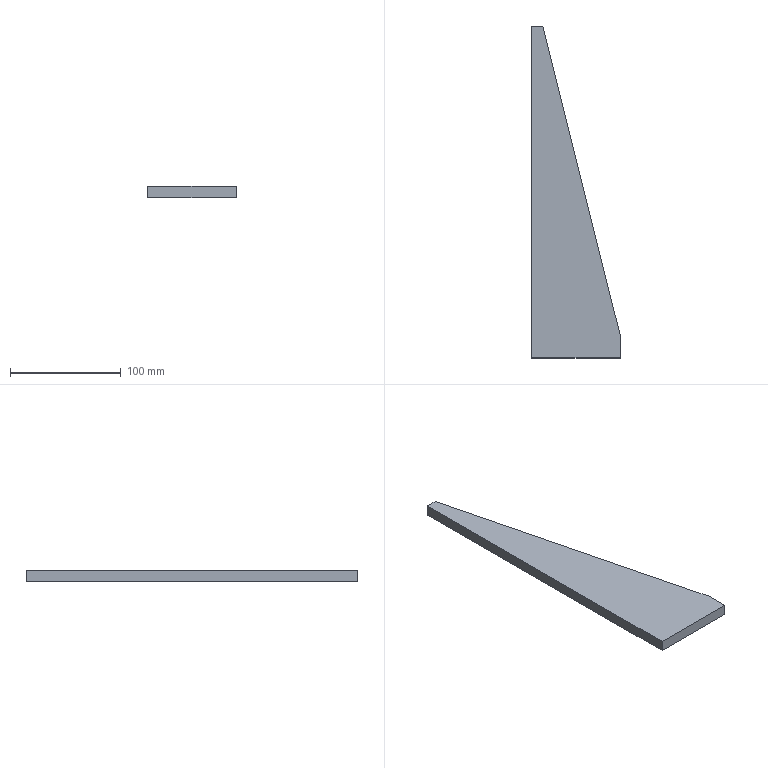Part | STEP file | 001-005-Shaft threading fixture rib plate | 1 solid | 7 faces | box 80 x 300 x 10 mm | volume 142000 mm3 | plane 7
STEP:
#1=CARTESIAN_POINT('',(0.,0.,0.));
#2=DIRECTION('',(0.,0.,1.));
#3=DIRECTION('',(1.,0.,0.));
#4=AXIS2_PLACEMENT_3D('',#1,#2,#3);
#5=CARTESIAN_POINT('',(40.,-150.,0.));
#6=VERTEX_POINT('',#5);
#7=CARTESIAN_POINT('',(40.,-130.,0.));
#8=VERTEX_POINT('',#7);
#9=CARTESIAN_POINT('',(40.,-150.,0.));
#10=DIRECTION('',(0.,1.,0.));
#11=VECTOR('',#10,1.);
#12=LINE('',#9,#11);
#13=CARTESIAN_POINT('',(40.,-150.,10.));
#14=DIRECTION('',(-1.,0.,0.));
#15=DIRECTION('',(0.,-1.,0.));
#16=AXIS2_PLACEMENT_3D('',#13,#14,#15);
#17=PLANE('',#16);
#18=CARTESIAN_POINT('',(0.,-10.));
#19=DIRECTION('',(-1.,0.));
#20=VECTOR('',#19,1.);
#21=LINE('',#18,#20);
#22=(GEOMETRIC_REPRESENTATION_CONTEXT(2)PARAMETRIC_REPRESENTATION_CONTEXT()REPRESENTATION_CONTEXT('',''));
#23=DEFINITIONAL_REPRESENTATION('',(#21),#22);
#24=PCURVE('',#17,#23);
#25=CARTESIAN_POINT('',(0.,0.,0.));
#26=DIRECTION('',(0.,0.,-1.));
#27=DIRECTION('',(-1.,0.,0.));
#28=AXIS2_PLACEMENT_3D('',#25,#26,#27);
#29=PLANE('',#28);
#30=CARTESIAN_POINT('',(-40.,-150.));
#31=DIRECTION('',(0.,1.));
#32=VECTOR('',#31,1.);
#33=LINE('',#30,#32);
#34=(GEOMETRIC_REPRESENTATION_CONTEXT(2)PARAMETRIC_REPRESENTATION_CONTEXT()REPRESENTATION_CONTEXT('',''));
#35=DEFINITIONAL_REPRESENTATION('',(#33),#34);
#36=PCURVE('',#29,#35);
#37=SURFACE_CURVE('',#12,(#24,#36),.PCURVE_S1.);
#38=EDGE_CURVE('',#6,#8,#37,.T.);
#39=ORIENTED_EDGE('',*,*,#38,.T.);
#40=CARTESIAN_POINT('',(40.,-130.,10.));
#41=VERTEX_POINT('',#40);
#42=CARTESIAN_POINT('',(40.,-130.,10.));
#43=DIRECTION('',(0.,0.,1.));
#44=VECTOR('',#43,1.);
#45=LINE('',#42,#44);
#46=CARTESIAN_POINT('',(-20.,0.));
#47=DIRECTION('',(0.,1.));
#48=VECTOR('',#47,1.);
#49=LINE('',#46,#48);
#50=(GEOMETRIC_REPRESENTATION_CONTEXT(2)PARAMETRIC_REPRESENTATION_CONTEXT()REPRESENTATION_CONTEXT('',''));
#51=DEFINITIONAL_REPRESENTATION('',(#49),#50);
#52=PCURVE('',#17,#51);
#53=CARTESIAN_POINT('',(-30.,150.,10.));
#54=DIRECTION('',(-0.9701,-0.2425,0.));
#55=DIRECTION('',(0.,0.,-1.));
#56=AXIS2_PLACEMENT_3D('',#53,#54,#55);
#57=PLANE('',#56);
#58=CARTESIAN_POINT('',(0.,288.617));
#59=DIRECTION('',(-1.,0.));
#60=VECTOR('',#59,1.);
#61=LINE('',#58,#60);
#62=(GEOMETRIC_REPRESENTATION_CONTEXT(2)PARAMETRIC_REPRESENTATION_CONTEXT()REPRESENTATION_CONTEXT('',''));
#63=DEFINITIONAL_REPRESENTATION('',(#61),#62);
#64=PCURVE('',#57,#63);
#65=SURFACE_CURVE('',#45,(#52,#64),.PCURVE_S1.);
#66=EDGE_CURVE('',#8,#41,#65,.T.);
#67=ORIENTED_EDGE('',*,*,#66,.T.);
#68=CARTESIAN_POINT('',(40.,-150.,10.));
#69=VERTEX_POINT('',#68);
#70=CARTESIAN_POINT('',(40.,-150.,10.));
#71=DIRECTION('',(0.,1.,0.));
#72=VECTOR('',#71,1.);
#73=LINE('',#70,#72);
#74=CARTESIAN_POINT('',(0.,0.));
#75=DIRECTION('',(-1.,0.));
#76=VECTOR('',#75,1.);
#77=LINE('',#74,#76);
#78=(GEOMETRIC_REPRESENTATION_CONTEXT(2)PARAMETRIC_REPRESENTATION_CONTEXT()REPRESENTATION_CONTEXT('',''));
#79=DEFINITIONAL_REPRESENTATION('',(#77),#78);
#80=PCURVE('',#17,#79);
#81=CARTESIAN_POINT('',(0.,0.,10.));
#82=DIRECTION('',(0.,0.,-1.));
#83=DIRECTION('',(-1.,0.,0.));
#84=AXIS2_PLACEMENT_3D('',#81,#82,#83);
#85=PLANE('',#84);
#86=CARTESIAN_POINT('',(-40.,-150.));
#87=DIRECTION('',(0.,1.));
#88=VECTOR('',#87,1.);
#89=LINE('',#86,#88);
#90=(GEOMETRIC_REPRESENTATION_CONTEXT(2)PARAMETRIC_REPRESENTATION_CONTEXT()REPRESENTATION_CONTEXT('',''));
#91=DEFINITIONAL_REPRESENTATION('',(#89),#90);
#92=PCURVE('',#85,#91);
#93=SURFACE_CURVE('',#73,(#80,#92),.PCURVE_S1.);
#94=EDGE_CURVE('',#69,#41,#93,.T.);
#95=ORIENTED_EDGE('',*,*,#94,.F.);
#96=CARTESIAN_POINT('',(40.,-150.,10.));
#97=DIRECTION('',(0.,0.,-1.));
#98=VECTOR('',#97,1.);
#99=LINE('',#96,#98);
#100=CARTESIAN_POINT('',(0.,0.));
#101=DIRECTION('',(0.,-1.));
#102=VECTOR('',#101,1.);
#103=LINE('',#100,#102);
#104=(GEOMETRIC_REPRESENTATION_CONTEXT(2)PARAMETRIC_REPRESENTATION_CONTEXT()REPRESENTATION_CONTEXT('',''));
#105=DEFINITIONAL_REPRESENTATION('',(#103),#104);
#106=PCURVE('',#17,#105);
#107=CARTESIAN_POINT('',(-40.,-150.,10.));
#108=DIRECTION('',(0.,1.,0.));
#109=DIRECTION('',(0.,0.,1.));
#110=AXIS2_PLACEMENT_3D('',#107,#108,#109);
#111=PLANE('',#110);
#112=CARTESIAN_POINT('',(0.,80.));
#113=DIRECTION('',(-1.,0.));
#114=VECTOR('',#113,1.);
#115=LINE('',#112,#114);
#116=(GEOMETRIC_REPRESENTATION_CONTEXT(2)PARAMETRIC_REPRESENTATION_CONTEXT()REPRESENTATION_CONTEXT('',''));
#117=DEFINITIONAL_REPRESENTATION('',(#115),#116);
#118=PCURVE('',#111,#117);
#119=SURFACE_CURVE('',#99,(#106,#118),.PCURVE_S1.);
#120=EDGE_CURVE('',#69,#6,#119,.T.);
#121=ORIENTED_EDGE('',*,*,#120,.T.);
#122=EDGE_LOOP('',(#39,#67,#95,#121));
#123=FACE_BOUND('',#122,.T.);
#124=ADVANCED_FACE('',(#123),#17,.F.);
#125=CARTESIAN_POINT('',(-30.,150.,10.));
#126=VERTEX_POINT('',#125);
#127=CARTESIAN_POINT('',(-40.,150.,10.));
#128=VERTEX_POINT('',#127);
#129=CARTESIAN_POINT('',(-40.,150.,10.));
#130=DIRECTION('',(-1.,0.,0.));
#131=VECTOR('',#130,1.);
#132=LINE('',#129,#131);
#133=CARTESIAN_POINT('',(-40.,150.,10.));
#134=DIRECTION('',(0.,-1.,0.));
#135=DIRECTION('',(1.,0.,0.));
#136=AXIS2_PLACEMENT_3D('',#133,#134,#135);
#137=PLANE('',#136);
#138=CARTESIAN_POINT('',(0.,0.));
#139=DIRECTION('',(-1.,0.));
#140=VECTOR('',#139,1.);
#141=LINE('',#138,#140);
#142=(GEOMETRIC_REPRESENTATION_CONTEXT(2)PARAMETRIC_REPRESENTATION_CONTEXT()REPRESENTATION_CONTEXT('',''));
#143=DEFINITIONAL_REPRESENTATION('',(#141),#142);
#144=PCURVE('',#137,#143);
#145=CARTESIAN_POINT('',(40.,150.));
#146=DIRECTION('',(1.,0.));
#147=VECTOR('',#146,1.);
#148=LINE('',#145,#147);
#149=(GEOMETRIC_REPRESENTATION_CONTEXT(2)PARAMETRIC_REPRESENTATION_CONTEXT()REPRESENTATION_CONTEXT('',''));
#150=DEFINITIONAL_REPRESENTATION('',(#148),#149);
#151=PCURVE('',#85,#150);
#152=SURFACE_CURVE('',#132,(#144,#151),.PCURVE_S1.);
#153=EDGE_CURVE('',#126,#128,#152,.T.);
#154=ORIENTED_EDGE('',*,*,#153,.F.);
#155=CARTESIAN_POINT('',(-30.,150.,0.));
#156=VERTEX_POINT('',#155);
#157=CARTESIAN_POINT('',(-30.,150.,10.));
#158=DIRECTION('',(0.,0.,-1.));
#159=VECTOR('',#158,1.);
#160=LINE('',#157,#159);
#161=CARTESIAN_POINT('',(10.,0.));
#162=DIRECTION('',(0.,-1.));
#163=VECTOR('',#162,1.);
#164=LINE('',#161,#163);
#165=(GEOMETRIC_REPRESENTATION_CONTEXT(2)PARAMETRIC_REPRESENTATION_CONTEXT()REPRESENTATION_CONTEXT('',''));
#166=DEFINITIONAL_REPRESENTATION('',(#164),#165);
#167=PCURVE('',#137,#166);
#168=CARTESIAN_POINT('',(0.,0.));
#169=DIRECTION('',(1.,0.));
#170=VECTOR('',#169,1.);
#171=LINE('',#168,#170);
#172=(GEOMETRIC_REPRESENTATION_CONTEXT(2)PARAMETRIC_REPRESENTATION_CONTEXT()REPRESENTATION_CONTEXT('',''));
#173=DEFINITIONAL_REPRESENTATION('',(#171),#172);
#174=PCURVE('',#57,#173);
#175=SURFACE_CURVE('',#160,(#167,#174),.PCURVE_S1.);
#176=EDGE_CURVE('',#126,#156,#175,.T.);
#177=ORIENTED_EDGE('',*,*,#176,.T.);
#178=CARTESIAN_POINT('',(-40.,150.,0.));
#179=VERTEX_POINT('',#178);
#180=CARTESIAN_POINT('',(-40.,150.,0.));
#181=DIRECTION('',(-1.,0.,0.));
#182=VECTOR('',#181,1.);
#183=LINE('',#180,#182);
#184=CARTESIAN_POINT('',(0.,-10.));
#185=DIRECTION('',(-1.,0.));
#186=VECTOR('',#185,1.);
#187=LINE('',#184,#186);
#188=(GEOMETRIC_REPRESENTATION_CONTEXT(2)PARAMETRIC_REPRESENTATION_CONTEXT()REPRESENTATION_CONTEXT('',''));
#189=DEFINITIONAL_REPRESENTATION('',(#187),#188);
#190=PCURVE('',#137,#189);
#191=CARTESIAN_POINT('',(40.,150.));
#192=DIRECTION('',(1.,0.));
#193=VECTOR('',#192,1.);
#194=LINE('',#191,#193);
#195=(GEOMETRIC_REPRESENTATION_CONTEXT(2)PARAMETRIC_REPRESENTATION_CONTEXT()REPRESENTATION_CONTEXT('',''));
#196=DEFINITIONAL_REPRESENTATION('',(#194),#195);
#197=PCURVE('',#29,#196);
#198=SURFACE_CURVE('',#183,(#190,#197),.PCURVE_S1.);
#199=EDGE_CURVE('',#156,#179,#198,.T.);
#200=ORIENTED_EDGE('',*,*,#199,.T.);
#201=CARTESIAN_POINT('',(-40.,150.,10.));
#202=DIRECTION('',(0.,0.,-1.));
#203=VECTOR('',#202,1.);
#204=LINE('',#201,#203);
#205=CARTESIAN_POINT('',(0.,0.));
#206=DIRECTION('',(0.,-1.));
#207=VECTOR('',#206,1.);
#208=LINE('',#205,#207);
#209=(GEOMETRIC_REPRESENTATION_CONTEXT(2)PARAMETRIC_REPRESENTATION_CONTEXT()REPRESENTATION_CONTEXT('',''));
#210=DEFINITIONAL_REPRESENTATION('',(#208),#209);
#211=PCURVE('',#137,#210);
#212=CARTESIAN_POINT('',(-40.,-150.,10.));
#213=DIRECTION('',(1.,0.,0.));
#214=DIRECTION('',(0.,1.,0.));
#215=AXIS2_PLACEMENT_3D('',#212,#213,#214);
#216=PLANE('',#215);
#217=CARTESIAN_POINT('',(300.,0.));
#218=DIRECTION('',(0.,-1.));
#219=VECTOR('',#218,1.);
#220=LINE('',#217,#219);
#221=(GEOMETRIC_REPRESENTATION_CONTEXT(2)PARAMETRIC_REPRESENTATION_CONTEXT()REPRESENTATION_CONTEXT('',''));
#222=DEFINITIONAL_REPRESENTATION('',(#220),#221);
#223=PCURVE('',#216,#222);
#224=SURFACE_CURVE('',#204,(#211,#223),.PCURVE_S1.);
#225=EDGE_CURVE('',#128,#179,#224,.T.);
#226=ORIENTED_EDGE('',*,*,#225,.F.);
#227=EDGE_LOOP('',(#154,#177,#200,#226));
#228=FACE_BOUND('',#227,.T.);
#229=ADVANCED_FACE('',(#228),#137,.F.);
#230=CARTESIAN_POINT('',(-40.,-150.,0.));
#231=VERTEX_POINT('',#230);
#232=CARTESIAN_POINT('',(-40.,-150.,0.));
#233=DIRECTION('',(0.,-1.,0.));
#234=VECTOR('',#233,1.);
#235=LINE('',#232,#234);
#236=CARTESIAN_POINT('',(0.,-10.));
#237=DIRECTION('',(-1.,0.));
#238=VECTOR('',#237,1.);
#239=LINE('',#236,#238);
#240=(GEOMETRIC_REPRESENTATION_CONTEXT(2)PARAMETRIC_REPRESENTATION_CONTEXT()REPRESENTATION_CONTEXT('',''));
#241=DEFINITIONAL_REPRESENTATION('',(#239),#240);
#242=PCURVE('',#216,#241);
#243=CARTESIAN_POINT('',(40.,-150.));
#244=DIRECTION('',(0.,-1.));
#245=VECTOR('',#244,1.);
#246=LINE('',#243,#245);
#247=(GEOMETRIC_REPRESENTATION_CONTEXT(2)PARAMETRIC_REPRESENTATION_CONTEXT()REPRESENTATION_CONTEXT('',''));
#248=DEFINITIONAL_REPRESENTATION('',(#246),#247);
#249=PCURVE('',#29,#248);
#250=SURFACE_CURVE('',#235,(#242,#249),.PCURVE_S1.);
#251=EDGE_CURVE('',#179,#231,#250,.T.);
#252=ORIENTED_EDGE('',*,*,#251,.T.);
#253=CARTESIAN_POINT('',(-40.,-150.,10.));
#254=VERTEX_POINT('',#253);
#255=CARTESIAN_POINT('',(-40.,-150.,10.));
#256=DIRECTION('',(0.,0.,-1.));
#257=VECTOR('',#256,1.);
#258=LINE('',#255,#257);
#259=CARTESIAN_POINT('',(0.,0.));
#260=DIRECTION('',(0.,-1.));
#261=VECTOR('',#260,1.);
#262=LINE('',#259,#261);
#263=(GEOMETRIC_REPRESENTATION_CONTEXT(2)PARAMETRIC_REPRESENTATION_CONTEXT()REPRESENTATION_CONTEXT('',''));
#264=DEFINITIONAL_REPRESENTATION('',(#262),#263);
#265=PCURVE('',#216,#264);
#266=CARTESIAN_POINT('',(0.,0.));
#267=DIRECTION('',(-1.,0.));
#268=VECTOR('',#267,1.);
#269=LINE('',#266,#268);
#270=(GEOMETRIC_REPRESENTATION_CONTEXT(2)PARAMETRIC_REPRESENTATION_CONTEXT()REPRESENTATION_CONTEXT('',''));
#271=DEFINITIONAL_REPRESENTATION('',(#269),#270);
#272=PCURVE('',#111,#271);
#273=SURFACE_CURVE('',#258,(#265,#272),.PCURVE_S1.);
#274=EDGE_CURVE('',#254,#231,#273,.T.);
#275=ORIENTED_EDGE('',*,*,#274,.F.);
#276=CARTESIAN_POINT('',(-40.,-150.,10.));
#277=DIRECTION('',(0.,-1.,0.));
#278=VECTOR('',#277,1.);
#279=LINE('',#276,#278);
#280=CARTESIAN_POINT('',(0.,0.));
#281=DIRECTION('',(-1.,0.));
#282=VECTOR('',#281,1.);
#283=LINE('',#280,#282);
#284=(GEOMETRIC_REPRESENTATION_CONTEXT(2)PARAMETRIC_REPRESENTATION_CONTEXT()REPRESENTATION_CONTEXT('',''));
#285=DEFINITIONAL_REPRESENTATION('',(#283),#284);
#286=PCURVE('',#216,#285);
#287=CARTESIAN_POINT('',(40.,-150.));
#288=DIRECTION('',(0.,-1.));
#289=VECTOR('',#288,1.);
#290=LINE('',#287,#289);
#291=(GEOMETRIC_REPRESENTATION_CONTEXT(2)PARAMETRIC_REPRESENTATION_CONTEXT()REPRESENTATION_CONTEXT('',''));
#292=DEFINITIONAL_REPRESENTATION('',(#290),#291);
#293=PCURVE('',#85,#292);
#294=SURFACE_CURVE('',#279,(#286,#293),.PCURVE_S1.);
#295=EDGE_CURVE('',#128,#254,#294,.T.);
#296=ORIENTED_EDGE('',*,*,#295,.F.);
#297=ORIENTED_EDGE('',*,*,#225,.T.);
#298=EDGE_LOOP('',(#252,#275,#296,#297));
#299=FACE_BOUND('',#298,.T.);
#300=ADVANCED_FACE('',(#299),#216,.F.);
#301=CARTESIAN_POINT('',(-40.,-150.,0.));
#302=DIRECTION('',(1.,0.,0.));
#303=VECTOR('',#302,1.);
#304=LINE('',#301,#303);
#305=CARTESIAN_POINT('',(-10.,0.));
#306=DIRECTION('',(0.,1.));
#307=VECTOR('',#306,1.);
#308=LINE('',#305,#307);
#309=(GEOMETRIC_REPRESENTATION_CONTEXT(2)PARAMETRIC_REPRESENTATION_CONTEXT()REPRESENTATION_CONTEXT('',''));
#310=DEFINITIONAL_REPRESENTATION('',(#308),#309);
#311=PCURVE('',#111,#310);
#312=CARTESIAN_POINT('',(40.,-150.));
#313=DIRECTION('',(-1.,0.));
#314=VECTOR('',#313,1.);
#315=LINE('',#312,#314);
#316=(GEOMETRIC_REPRESENTATION_CONTEXT(2)PARAMETRIC_REPRESENTATION_CONTEXT()REPRESENTATION_CONTEXT('',''));
#317=DEFINITIONAL_REPRESENTATION('',(#315),#316);
#318=PCURVE('',#29,#317);
#319=SURFACE_CURVE('',#304,(#311,#318),.PCURVE_S1.);
#320=EDGE_CURVE('',#231,#6,#319,.T.);
#321=ORIENTED_EDGE('',*,*,#320,.T.);
#322=ORIENTED_EDGE('',*,*,#120,.F.);
#323=CARTESIAN_POINT('',(-40.,-150.,10.));
#324=DIRECTION('',(1.,0.,0.));
#325=VECTOR('',#324,1.);
#326=LINE('',#323,#325);
#327=CARTESIAN_POINT('',(0.,0.));
#328=DIRECTION('',(0.,1.));
#329=VECTOR('',#328,1.);
#330=LINE('',#327,#329);
#331=(GEOMETRIC_REPRESENTATION_CONTEXT(2)PARAMETRIC_REPRESENTATION_CONTEXT()REPRESENTATION_CONTEXT('',''));
#332=DEFINITIONAL_REPRESENTATION('',(#330),#331);
#333=PCURVE('',#111,#332);
#334=CARTESIAN_POINT('',(40.,-150.));
#335=DIRECTION('',(-1.,0.));
#336=VECTOR('',#335,1.);
#337=LINE('',#334,#336);
#338=(GEOMETRIC_REPRESENTATION_CONTEXT(2)PARAMETRIC_REPRESENTATION_CONTEXT()REPRESENTATION_CONTEXT('',''));
#339=DEFINITIONAL_REPRESENTATION('',(#337),#338);
#340=PCURVE('',#85,#339);
#341=SURFACE_CURVE('',#326,(#333,#340),.PCURVE_S1.);
#342=EDGE_CURVE('',#254,#69,#341,.T.);
#343=ORIENTED_EDGE('',*,*,#342,.F.);
#344=ORIENTED_EDGE('',*,*,#274,.T.);
#345=EDGE_LOOP('',(#321,#322,#343,#344));
#346=FACE_BOUND('',#345,.T.);
#347=ADVANCED_FACE('',(#346),#111,.F.);
#348=ORIENTED_EDGE('',*,*,#94,.T.);
#349=CARTESIAN_POINT('',(-30.,150.,10.));
#350=DIRECTION('',(-0.2425,0.9701,0.));
#351=VECTOR('',#350,1.);
#352=LINE('',#349,#351);
#353=CARTESIAN_POINT('',(30.,150.));
#354=DIRECTION('',(0.2425,0.9701));
#355=VECTOR('',#354,1.);
#356=LINE('',#353,#355);
#357=(GEOMETRIC_REPRESENTATION_CONTEXT(2)PARAMETRIC_REPRESENTATION_CONTEXT()REPRESENTATION_CONTEXT('',''));
#358=DEFINITIONAL_REPRESENTATION('',(#356),#357);
#359=PCURVE('',#85,#358);
#360=CARTESIAN_POINT('',(0.,0.));
#361=DIRECTION('',(0.,-1.));
#362=VECTOR('',#361,1.);
#363=LINE('',#360,#362);
#364=(GEOMETRIC_REPRESENTATION_CONTEXT(2)PARAMETRIC_REPRESENTATION_CONTEXT()REPRESENTATION_CONTEXT('',''));
#365=DEFINITIONAL_REPRESENTATION('',(#363),#364);
#366=PCURVE('',#57,#365);
#367=SURFACE_CURVE('',#352,(#359,#366),.PCURVE_S1.);
#368=EDGE_CURVE('',#41,#126,#367,.T.);
#369=ORIENTED_EDGE('',*,*,#368,.T.);
#370=ORIENTED_EDGE('',*,*,#153,.T.);
#371=ORIENTED_EDGE('',*,*,#295,.T.);
#372=ORIENTED_EDGE('',*,*,#342,.T.);
#373=EDGE_LOOP('',(#348,#369,#370,#371,#372));
#374=FACE_BOUND('',#373,.T.);
#375=ADVANCED_FACE('',(#374),#85,.F.);
#376=ORIENTED_EDGE('',*,*,#199,.F.);
#377=CARTESIAN_POINT('',(7.059,1.765,0.));
#378=DIRECTION('',(0.2425,-0.9701,0.));
#379=VECTOR('',#378,1.);
#380=LINE('',#377,#379);
#381=CARTESIAN_POINT('',(-7.059,1.765));
#382=DIRECTION('',(-0.2425,-0.9701));
#383=VECTOR('',#382,1.);
#384=LINE('',#381,#383);
#385=(GEOMETRIC_REPRESENTATION_CONTEXT(2)PARAMETRIC_REPRESENTATION_CONTEXT()REPRESENTATION_CONTEXT('',''));
#386=DEFINITIONAL_REPRESENTATION('',(#384),#385);
#387=PCURVE('',#29,#386);
#388=CARTESIAN_POINT('',(10.,152.797));
#389=DIRECTION('',(0.,1.));
#390=VECTOR('',#389,1.);
#391=LINE('',#388,#390);
#392=(GEOMETRIC_REPRESENTATION_CONTEXT(2)PARAMETRIC_REPRESENTATION_CONTEXT()REPRESENTATION_CONTEXT('',''));
#393=DEFINITIONAL_REPRESENTATION('',(#391),#392);
#394=PCURVE('',#57,#393);
#395=SURFACE_CURVE('',#380,(#387,#394),.PCURVE_S1.);
#396=EDGE_CURVE('',#156,#8,#395,.T.);
#397=ORIENTED_EDGE('',*,*,#396,.T.);
#398=ORIENTED_EDGE('',*,*,#38,.F.);
#399=ORIENTED_EDGE('',*,*,#320,.F.);
#400=ORIENTED_EDGE('',*,*,#251,.F.);
#401=EDGE_LOOP('',(#376,#397,#398,#399,#400));
#402=FACE_BOUND('',#401,.T.);
#403=ADVANCED_FACE('',(#402),#29,.T.);
#404=ORIENTED_EDGE('',*,*,#368,.F.);
#405=ORIENTED_EDGE('',*,*,#66,.F.);
#406=ORIENTED_EDGE('',*,*,#396,.F.);
#407=ORIENTED_EDGE('',*,*,#176,.F.);
#408=EDGE_LOOP('',(#404,#405,#406,#407));
#409=FACE_BOUND('',#408,.T.);
#410=ADVANCED_FACE('',(#409),#57,.F.);
#411=CLOSED_SHELL('',(#124,#229,#300,#347,#375,#403,#410));
#412=MANIFOLD_SOLID_BREP('',#411);
#413=(LENGTH_UNIT()NAMED_UNIT(*)SI_UNIT(.MILLI.,.METRE.));
#414=UNCERTAINTY_MEASURE_WITH_UNIT(LENGTH_MEASURE(0.0000001),#413,'','');
#415=(NAMED_UNIT(*)PLANE_ANGLE_UNIT()SI_UNIT($,.RADIAN.));
#416=(NAMED_UNIT(*)SI_UNIT($,.STERADIAN.)SOLID_ANGLE_UNIT());
#417=(GEOMETRIC_REPRESENTATION_CONTEXT(3)GLOBAL_UNCERTAINTY_ASSIGNED_CONTEXT((#414))GLOBAL_UNIT_ASSIGNED_CONTEXT((#413,#415,#416))REPRESENTATION_CONTEXT('',''));
#418=ADVANCED_BREP_SHAPE_REPRESENTATION('',(#4,#412),#417);